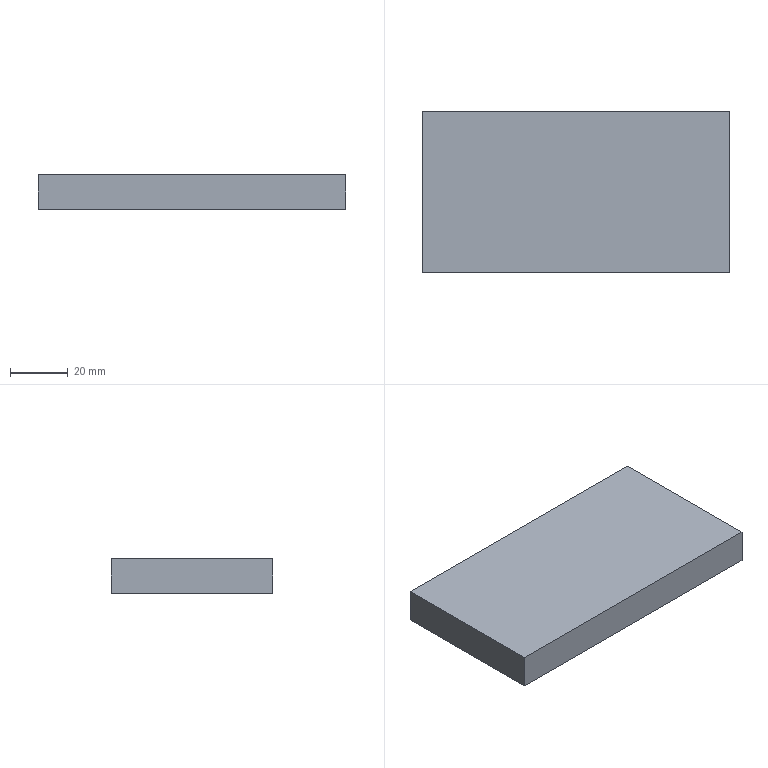Part | STEP file | Part 19^PN_0001_ASM-2 | 1 solid | 6 faces | box 106.46 x 56 x 12 mm | volume 71541 mm3 | plane 6
STEP:
#1=CARTESIAN_POINT('',(171.087,15.,0.));
#2=VERTEX_POINT('',#1);
#3=CARTESIAN_POINT('',(171.087,-41.,0.));
#4=VERTEX_POINT('',#3);
#5=CARTESIAN_POINT('',(171.087,15.,0.));
#6=DIRECTION('',(0.,-1.,0.));
#7=VECTOR('',#6,1000.);
#8=LINE('',#5,#7);
#9=EDGE_CURVE('',#2,#4,#8,.T.);
#10=ORIENTED_EDGE('',*,*,#9,.T.);
#11=CARTESIAN_POINT('',(171.087,-41.,12.));
#12=VERTEX_POINT('',#11);
#13=CARTESIAN_POINT('',(171.087,-41.,12.));
#14=DIRECTION('',(0.,0.,-1.));
#15=VECTOR('',#14,1000.);
#16=LINE('',#13,#15);
#17=EDGE_CURVE('',#12,#4,#16,.T.);
#18=ORIENTED_EDGE('',*,*,#17,.F.);
#19=CARTESIAN_POINT('',(171.087,15.,12.));
#20=VERTEX_POINT('',#19);
#21=CARTESIAN_POINT('',(171.087,15.,12.));
#22=DIRECTION('',(0.,-1.,0.));
#23=VECTOR('',#22,1000.);
#24=LINE('',#21,#23);
#25=EDGE_CURVE('',#20,#12,#24,.T.);
#26=ORIENTED_EDGE('',*,*,#25,.F.);
#27=CARTESIAN_POINT('',(171.087,15.,12.));
#28=DIRECTION('',(0.,0.,-1.));
#29=VECTOR('',#28,1000.);
#30=LINE('',#27,#29);
#31=EDGE_CURVE('',#20,#2,#30,.T.);
#32=ORIENTED_EDGE('',*,*,#31,.T.);
#33=EDGE_LOOP('',(#10,#18,#26,#32));
#34=FACE_OUTER_BOUND('',#33,.T.);
#35=CARTESIAN_POINT('',(171.087,15.,12.));
#36=DIRECTION('',(1.,0.,0.));
#37=DIRECTION('',(0.,0.,-1.));
#38=AXIS2_PLACEMENT_3D('',#35,#36,#37);
#39=PLANE('',#38);
#40=ADVANCED_FACE('',(#34),#39,.F.);
#41=CARTESIAN_POINT('',(277.547,-41.,0.));
#42=VERTEX_POINT('',#41);
#43=CARTESIAN_POINT('',(171.087,-41.,0.));
#44=DIRECTION('',(1.,0.,0.));
#45=VECTOR('',#44,1000.);
#46=LINE('',#43,#45);
#47=EDGE_CURVE('',#4,#42,#46,.T.);
#48=ORIENTED_EDGE('',*,*,#47,.T.);
#49=CARTESIAN_POINT('',(277.547,-41.,12.));
#50=VERTEX_POINT('',#49);
#51=CARTESIAN_POINT('',(277.547,-41.,12.));
#52=DIRECTION('',(0.,0.,-1.));
#53=VECTOR('',#52,1000.);
#54=LINE('',#51,#53);
#55=EDGE_CURVE('',#50,#42,#54,.T.);
#56=ORIENTED_EDGE('',*,*,#55,.F.);
#57=CARTESIAN_POINT('',(171.087,-41.,12.));
#58=DIRECTION('',(1.,0.,0.));
#59=VECTOR('',#58,1000.);
#60=LINE('',#57,#59);
#61=EDGE_CURVE('',#12,#50,#60,.T.);
#62=ORIENTED_EDGE('',*,*,#61,.F.);
#63=ORIENTED_EDGE('',*,*,#17,.T.);
#64=EDGE_LOOP('',(#48,#56,#62,#63));
#65=FACE_OUTER_BOUND('',#64,.T.);
#66=CARTESIAN_POINT('',(171.087,-41.,12.));
#67=DIRECTION('',(0.,1.,0.));
#68=DIRECTION('',(0.,0.,1.));
#69=AXIS2_PLACEMENT_3D('',#66,#67,#68);
#70=PLANE('',#69);
#71=ADVANCED_FACE('',(#65),#70,.F.);
#72=CARTESIAN_POINT('',(277.547,15.,0.));
#73=VERTEX_POINT('',#72);
#74=CARTESIAN_POINT('',(277.547,15.,0.));
#75=DIRECTION('',(0.,1.,0.));
#76=VECTOR('',#75,1000.);
#77=LINE('',#74,#76);
#78=EDGE_CURVE('',#42,#73,#77,.T.);
#79=ORIENTED_EDGE('',*,*,#78,.T.);
#80=CARTESIAN_POINT('',(277.547,15.,12.));
#81=VERTEX_POINT('',#80);
#82=CARTESIAN_POINT('',(277.547,15.,12.));
#83=DIRECTION('',(0.,0.,-1.));
#84=VECTOR('',#83,1000.);
#85=LINE('',#82,#84);
#86=EDGE_CURVE('',#81,#73,#85,.T.);
#87=ORIENTED_EDGE('',*,*,#86,.F.);
#88=CARTESIAN_POINT('',(277.547,15.,12.));
#89=DIRECTION('',(0.,1.,0.));
#90=VECTOR('',#89,1000.);
#91=LINE('',#88,#90);
#92=EDGE_CURVE('',#50,#81,#91,.T.);
#93=ORIENTED_EDGE('',*,*,#92,.F.);
#94=ORIENTED_EDGE('',*,*,#55,.T.);
#95=EDGE_LOOP('',(#79,#87,#93,#94));
#96=FACE_OUTER_BOUND('',#95,.T.);
#97=CARTESIAN_POINT('',(277.547,15.,12.));
#98=DIRECTION('',(-1.,0.,0.));
#99=DIRECTION('',(0.,0.,1.));
#100=AXIS2_PLACEMENT_3D('',#97,#98,#99);
#101=PLANE('',#100);
#102=ADVANCED_FACE('',(#96),#101,.F.);
#103=CARTESIAN_POINT('',(171.087,15.,0.));
#104=DIRECTION('',(-1.,0.,0.));
#105=VECTOR('',#104,1000.);
#106=LINE('',#103,#105);
#107=EDGE_CURVE('',#73,#2,#106,.T.);
#108=ORIENTED_EDGE('',*,*,#107,.T.);
#109=ORIENTED_EDGE('',*,*,#31,.F.);
#110=CARTESIAN_POINT('',(171.087,15.,12.));
#111=DIRECTION('',(-1.,0.,0.));
#112=VECTOR('',#111,1000.);
#113=LINE('',#110,#112);
#114=EDGE_CURVE('',#81,#20,#113,.T.);
#115=ORIENTED_EDGE('',*,*,#114,.F.);
#116=ORIENTED_EDGE('',*,*,#86,.T.);
#117=EDGE_LOOP('',(#108,#109,#115,#116));
#118=FACE_OUTER_BOUND('',#117,.T.);
#119=CARTESIAN_POINT('',(171.087,15.,12.));
#120=DIRECTION('',(0.,-1.,0.));
#121=DIRECTION('',(0.,0.,-1.));
#122=AXIS2_PLACEMENT_3D('',#119,#120,#121);
#123=PLANE('',#122);
#124=ADVANCED_FACE('',(#118),#123,.F.);
#125=ORIENTED_EDGE('',*,*,#25,.T.);
#126=ORIENTED_EDGE('',*,*,#61,.T.);
#127=ORIENTED_EDGE('',*,*,#92,.T.);
#128=ORIENTED_EDGE('',*,*,#114,.T.);
#129=EDGE_LOOP('',(#125,#126,#127,#128));
#130=FACE_OUTER_BOUND('',#129,.T.);
#131=CARTESIAN_POINT('',(171.087,-41.,12.));
#132=DIRECTION('',(0.,0.,1.));
#133=DIRECTION('',(1.,0.,0.));
#134=AXIS2_PLACEMENT_3D('',#131,#132,#133);
#135=PLANE('',#134);
#136=ADVANCED_FACE('',(#130),#135,.T.);
#137=ORIENTED_EDGE('',*,*,#9,.F.);
#138=ORIENTED_EDGE('',*,*,#107,.F.);
#139=ORIENTED_EDGE('',*,*,#78,.F.);
#140=ORIENTED_EDGE('',*,*,#47,.F.);
#141=EDGE_LOOP('',(#137,#138,#139,#140));
#142=FACE_OUTER_BOUND('',#141,.T.);
#143=CARTESIAN_POINT('',(171.087,-41.,0.));
#144=DIRECTION('',(0.,0.,1.));
#145=DIRECTION('',(1.,0.,0.));
#146=AXIS2_PLACEMENT_3D('',#143,#144,#145);
#147=PLANE('',#146);
#148=ADVANCED_FACE('',(#142),#147,.F.);
#149=CLOSED_SHELL('',(#40,#71,#102,#124,#136,#148));
#150=MANIFOLD_SOLID_BREP('',#149);
#151=CARTESIAN_POINT('',(0.,0.,0.));
#152=DIRECTION('',(0.,0.,1.));
#153=DIRECTION('',(1.,0.,0.));
#154=AXIS2_PLACEMENT_3D('',#151,#152,#153);
#155=(LENGTH_UNIT()NAMED_UNIT(*)SI_UNIT(.MILLI.,.METRE.));
#156=UNCERTAINTY_MEASURE_WITH_UNIT(LENGTH_MEASURE(0.00001),#155,'','');
#157=(NAMED_UNIT(*)PLANE_ANGLE_UNIT()SI_UNIT($,.RADIAN.));
#158=(NAMED_UNIT(*)SI_UNIT($,.STERADIAN.)SOLID_ANGLE_UNIT());
#159=(GEOMETRIC_REPRESENTATION_CONTEXT(3)GLOBAL_UNCERTAINTY_ASSIGNED_CONTEXT((#156))GLOBAL_UNIT_ASSIGNED_CONTEXT((#155,#157,#158))REPRESENTATION_CONTEXT('',''));
#160=ADVANCED_BREP_SHAPE_REPRESENTATION('',(#150,#154),#159);